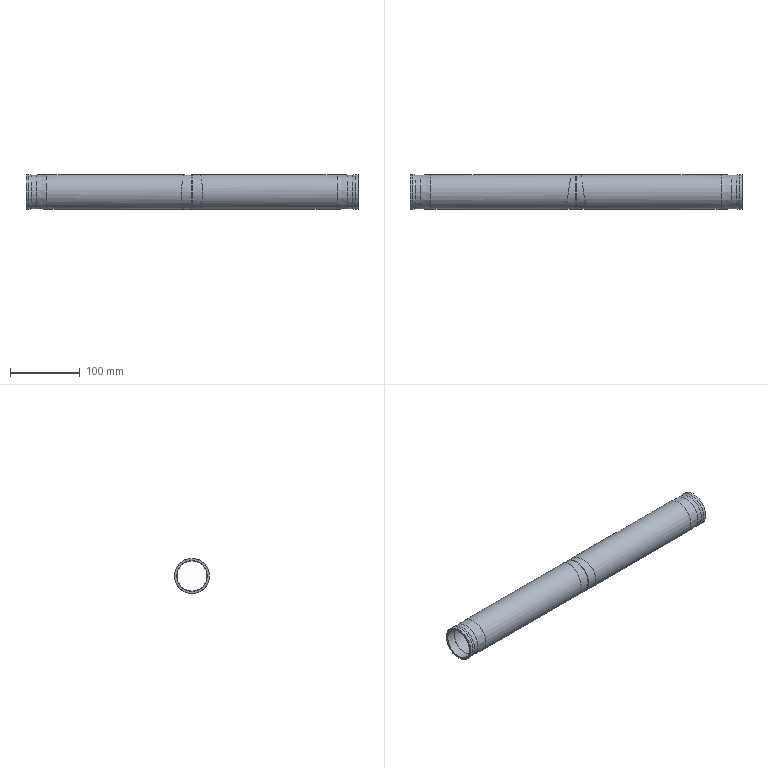Part | STEP file | 610B0801 | 1 solid | 20 faces | box 475 x 50 x 50 mm | volume 237316 mm3 | cylinder 12 | plane 4 | cone 4 | commonest cylinder face diameters 50 x7 44 x2 48.5 x2 43 x1